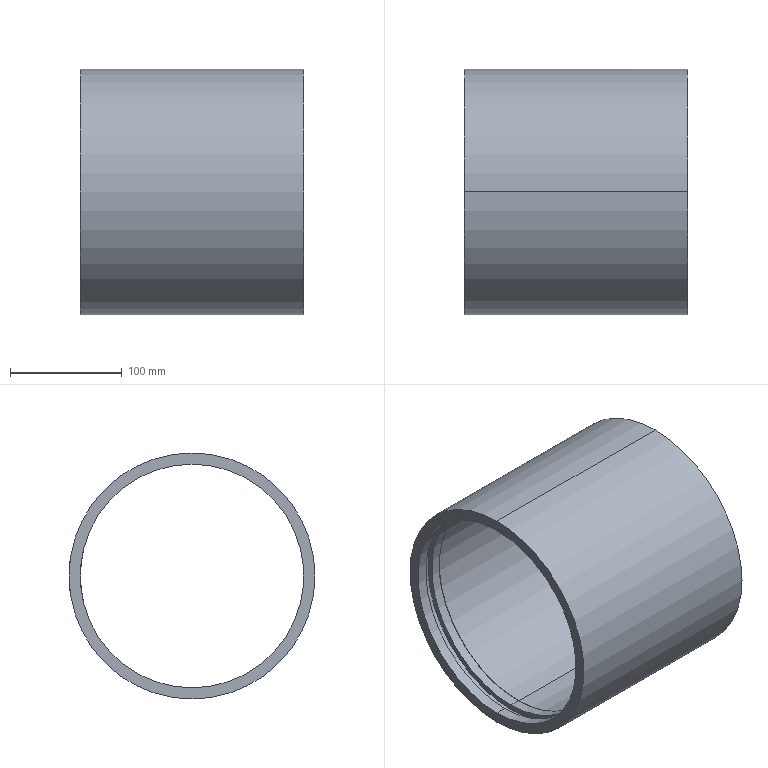Part | SolidWorks | features ICE 2, Revolution 1 | 1 solid | 23 faces | box 200 x 220 x 220 mm | volume 1255193 mm3 | cylinder 16 | plane 7 | commonest cylinder face diameters 200 x6 8.5 x2 14 x2 201 x2 210 x2 220 x2
STEP:
#1=CARTESIAN_POINT('',(106.5,99.91,-4.25));
#2=VERTEX_POINT('',#1);
#3=CARTESIAN_POINT('',(106.5,99.91,4.25));
#4=VERTEX_POINT('',#3);
#5=CARTESIAN_POINT('',(106.5,99.91,-4.25));
#6=CARTESIAN_POINT('',(106.223,99.91,-4.25));
#7=CARTESIAN_POINT('',(105.947,99.911,-4.223));
#8=CARTESIAN_POINT('',(105.399,99.915,-4.114));
#9=CARTESIAN_POINT('',(105.131,99.919,-4.033));
#10=CARTESIAN_POINT('',(104.619,99.927,-3.821));
#11=CARTESIAN_POINT('',(104.373,99.932,-3.69));
#12=CARTESIAN_POINT('',(103.907,99.943,-3.379));
#13=CARTESIAN_POINT('',(103.693,99.949,-3.203));
#14=CARTESIAN_POINT('',(103.301,99.961,-2.812));
#15=CARTESIAN_POINT('',(103.122,99.967,-2.593));
#16=CARTESIAN_POINT('',(102.813,99.978,-2.131));
#17=CARTESIAN_POINT('',(102.682,99.983,-1.887));
#18=CARTESIAN_POINT('',(102.469,99.991,-1.373));
#19=CARTESIAN_POINT('',(102.387,99.994,-1.103));
#20=CARTESIAN_POINT('',(102.278,99.999,-0.5597));
#21=CARTESIAN_POINT('',(102.25,100.,-0.2838));
#22=CARTESIAN_POINT('',(102.25,100.,0.2768));
#23=CARTESIAN_POINT('',(102.277,99.999,0.554));
#24=CARTESIAN_POINT('',(102.385,99.994,1.097));
#25=CARTESIAN_POINT('',(102.466,99.991,1.367));
#26=CARTESIAN_POINT('',(102.679,99.983,1.882));
#27=CARTESIAN_POINT('',(102.81,99.978,2.126));
#28=CARTESIAN_POINT('',(103.118,99.967,2.588));
#29=CARTESIAN_POINT('',(103.297,99.961,2.807));
#30=CARTESIAN_POINT('',(103.689,99.949,3.199));
#31=CARTESIAN_POINT('',(103.903,99.943,3.375));
#32=CARTESIAN_POINT('',(104.366,99.932,3.686));
#33=CARTESIAN_POINT('',(104.614,99.927,3.819));
#34=CARTESIAN_POINT('',(105.125,99.919,4.031));
#35=CARTESIAN_POINT('',(105.392,99.915,4.112));
#36=CARTESIAN_POINT('',(105.942,99.911,4.222));
#37=CARTESIAN_POINT('',(106.219,99.91,4.25));
#38=CARTESIAN_POINT('',(106.5,99.91,4.25));
#39=B_SPLINE_CURVE_WITH_KNOTS('',3,(#5,#6,#7,#8,#9,#10,#11,#12,#13,#14,#15,#16,#17,#18,#19,#20,#21,#22,#23,#24,#25,#26,#27,#28,#29,#30,#31,#32,#33,#34,#35,#36,#37,#38),.UNSPECIFIED.,.F.,.F.,(4,2,2,2,2,2,2,2,2,2,2,2,2,2,2,2,4),(0.01329,0.01412,0.01495,0.01578,0.01661,0.01744,0.01827,0.0191,0.01993,0.02076,0.02159,0.02242,0.02325,0.02408,0.02491,0.02574,0.02657),.UNSPECIFIED.);
#40=EDGE_CURVE('',#2,#4,#39,.T.);
#41=ORIENTED_EDGE('',*,*,#40,.F.);
#42=CARTESIAN_POINT('',(106.5,101.5,-4.25));
#43=VERTEX_POINT('',#42);
#44=CARTESIAN_POINT('',(106.5,93.,-4.25));
#45=DIRECTION('',(0.,1.,0.));
#46=VECTOR('',#45,1000.);
#47=LINE('',#44,#46);
#48=EDGE_CURVE('',#2,#43,#47,.T.);
#49=ORIENTED_EDGE('',*,*,#48,.T.);
#50=CARTESIAN_POINT('',(106.5,101.5,4.25));
#51=VERTEX_POINT('',#50);
#52=CARTESIAN_POINT('',(106.5,101.5,0.));
#53=DIRECTION('',(0.,1.,0.));
#54=DIRECTION('',(0.,0.,1.));
#55=AXIS2_PLACEMENT_3D('',#52,#53,#54);
#56=CIRCLE('',#55,4.25);
#57=EDGE_CURVE('',#43,#51,#56,.T.);
#58=ORIENTED_EDGE('',*,*,#57,.T.);
#59=CARTESIAN_POINT('',(106.5,93.,4.25));
#60=DIRECTION('',(0.,1.,0.));
#61=VECTOR('',#60,1000.);
#62=LINE('',#59,#61);
#63=EDGE_CURVE('',#4,#51,#62,.T.);
#64=ORIENTED_EDGE('',*,*,#63,.F.);
#65=EDGE_LOOP('',(#41,#49,#58,#64));
#66=FACE_OUTER_BOUND('',#65,.T.);
#67=CARTESIAN_POINT('',(106.5,93.,0.));
#68=DIRECTION('',(0.,1.,0.));
#69=DIRECTION('',(0.,0.,1.));
#70=AXIS2_PLACEMENT_3D('',#67,#68,#69);
#71=CYLINDRICAL_SURFACE('',#70,4.25);
#72=ADVANCED_FACE('',(#66),#71,.F.);
#73=CARTESIAN_POINT('',(106.5,101.5,-7.));
#74=VERTEX_POINT('',#73);
#75=CARTESIAN_POINT('',(106.5,101.5,7.));
#76=VERTEX_POINT('',#75);
#77=CARTESIAN_POINT('',(106.5,101.5,0.));
#78=DIRECTION('',(0.,1.,0.));
#79=DIRECTION('',(0.,0.,1.));
#80=AXIS2_PLACEMENT_3D('',#77,#78,#79);
#81=CIRCLE('',#80,7.);
#82=EDGE_CURVE('',#74,#76,#81,.T.);
#83=ORIENTED_EDGE('',*,*,#82,.F.);
#84=CARTESIAN_POINT('',(106.5,109.777,-7.));
#85=VERTEX_POINT('',#84);
#86=CARTESIAN_POINT('',(106.5,101.5,-7.));
#87=DIRECTION('',(0.,1.,0.));
#88=VECTOR('',#87,1000.);
#89=LINE('',#86,#88);
#90=EDGE_CURVE('',#74,#85,#89,.T.);
#91=ORIENTED_EDGE('',*,*,#90,.T.);
#92=CARTESIAN_POINT('',(106.5,109.777,7.));
#93=VERTEX_POINT('',#92);
#94=CARTESIAN_POINT('',(106.5,109.777,7.));
#95=CARTESIAN_POINT('',(106.038,109.777,7.));
#96=CARTESIAN_POINT('',(105.583,109.78,6.955));
#97=CARTESIAN_POINT('',(104.912,109.788,6.821));
#98=CARTESIAN_POINT('',(104.69,109.792,6.766));
#99=CARTESIAN_POINT('',(104.25,109.8,6.632));
#100=CARTESIAN_POINT('',(104.031,109.805,6.554));
#101=CARTESIAN_POINT('',(103.395,109.82,6.291));
#102=CARTESIAN_POINT('',(102.993,109.832,6.075));
#103=CARTESIAN_POINT('',(102.233,109.859,5.567));
#104=CARTESIAN_POINT('',(101.872,109.874,5.272));
#105=CARTESIAN_POINT('',(101.227,109.903,4.626));
#106=CARTESIAN_POINT('',(100.937,109.918,4.274));
#107=CARTESIAN_POINT('',(100.553,109.938,3.7));
#108=CARTESIAN_POINT('',(100.434,109.944,3.501));
#109=CARTESIAN_POINT('',(100.218,109.957,3.097));
#110=CARTESIAN_POINT('',(100.023,109.968,2.684));
#111=CARTESIAN_POINT('',(99.869,109.977,2.254));
#112=CARTESIAN_POINT('',(99.736,109.985,1.816));
#113=CARTESIAN_POINT('',(99.68,109.989,1.591));
#114=CARTESIAN_POINT('',(99.545,109.997,0.9135));
#115=CARTESIAN_POINT('',(99.5,110.,0.4592));
#116=CARTESIAN_POINT('',(99.5,110.,-0.4542));
#117=CARTESIAN_POINT('',(99.546,109.997,-0.9181));
#118=CARTESIAN_POINT('',(99.724,109.986,-1.816));
#119=CARTESIAN_POINT('',(99.857,109.978,-2.252));
#120=CARTESIAN_POINT('',(100.12,109.962,-2.888));
#121=CARTESIAN_POINT('',(100.219,109.957,-3.098));
#122=CARTESIAN_POINT('',(100.436,109.944,-3.503));
#123=CARTESIAN_POINT('',(100.553,109.938,-3.699));
#124=CARTESIAN_POINT('',(100.933,109.918,-4.268));
#125=CARTESIAN_POINT('',(101.223,109.903,-4.622));
#126=CARTESIAN_POINT('',(101.876,109.874,-5.276));
#127=CARTESIAN_POINT('',(102.23,109.859,-5.565));
#128=CARTESIAN_POINT('',(102.799,109.839,-5.946));
#129=CARTESIAN_POINT('',(102.995,109.833,-6.063));
#130=CARTESIAN_POINT('',(103.4,109.821,-6.28));
#131=CARTESIAN_POINT('',(103.609,109.815,-6.379));
#132=CARTESIAN_POINT('',(104.246,109.799,-6.643));
#133=CARTESIAN_POINT('',(104.682,109.791,-6.775));
#134=CARTESIAN_POINT('',(105.579,109.78,-6.954));
#135=CARTESIAN_POINT('',(106.043,109.777,-7.));
#136=CARTESIAN_POINT('',(106.5,109.777,-7.));
#137=B_SPLINE_CURVE_WITH_KNOTS('',3,(#94,#95,#96,#97,#98,#99,#100,#101,#102,#103,#104,#105,#106,#107,#108,#109,#110,#111,#112,#113,#114,#115,#116,#117,#118,#119,#120,#121,#122,#123,#124,#125,#126,#127,#128,#129,#130,#131,#132,#133,#134,#135,#136),.UNSPECIFIED.,.F.,.F.,(4,2,2,2,2,2,2,2,1,2,2,2,2,2,2,2,2,2,2,2,2,4),(0.,0.001368,0.002052,0.002736,0.004105,0.005473,0.006841,0.007525,0.008209,0.008893,0.009577,0.01095,0.01231,0.01368,0.01437,0.01505,0.01642,0.01779,0.01847,0.01915,0.02052,0.02189),.UNSPECIFIED.);
#138=EDGE_CURVE('',#93,#85,#137,.T.);
#139=ORIENTED_EDGE('',*,*,#138,.F.);
#140=CARTESIAN_POINT('',(106.5,101.5,7.));
#141=DIRECTION('',(0.,1.,0.));
#142=VECTOR('',#141,1000.);
#143=LINE('',#140,#142);
#144=EDGE_CURVE('',#76,#93,#143,.T.);
#145=ORIENTED_EDGE('',*,*,#144,.F.);
#146=EDGE_LOOP('',(#83,#91,#139,#145));
#147=FACE_OUTER_BOUND('',#146,.T.);
#148=CARTESIAN_POINT('',(106.5,101.5,0.));
#149=DIRECTION('',(0.,1.,0.));
#150=DIRECTION('',(0.,0.,1.));
#151=AXIS2_PLACEMENT_3D('',#148,#149,#150);
#152=CYLINDRICAL_SURFACE('',#151,7.);
#153=ADVANCED_FACE('',(#147),#152,.F.);
#154=CARTESIAN_POINT('',(-71.,0.,-100.));
#155=VERTEX_POINT('',#154);
#156=CARTESIAN_POINT('',(-71.,0.,100.));
#157=VERTEX_POINT('',#156);
#158=CARTESIAN_POINT('',(-71.,0.,0.));
#159=DIRECTION('',(-1.,0.,0.));
#160=DIRECTION('',(0.,0.,1.));
#161=AXIS2_PLACEMENT_3D('',#158,#159,#160);
#162=CIRCLE('',#161,100.);
#163=EDGE_CURVE('',#155,#157,#162,.T.);
#164=ORIENTED_EDGE('',*,*,#163,.F.);
#165=CARTESIAN_POINT('',(-81.,0.,-100.));
#166=VERTEX_POINT('',#165);
#167=CARTESIAN_POINT('',(-113.63,0.,-100.));
#168=DIRECTION('',(-1.,0.,0.));
#169=VECTOR('',#168,1000.);
#170=LINE('',#167,#169);
#171=EDGE_CURVE('',#155,#166,#170,.T.);
#172=ORIENTED_EDGE('',*,*,#171,.T.);
#173=CARTESIAN_POINT('',(-81.,0.,100.));
#174=VERTEX_POINT('',#173);
#175=CARTESIAN_POINT('',(-81.,0.,0.));
#176=DIRECTION('',(-1.,0.,0.));
#177=DIRECTION('',(0.,0.,1.));
#178=AXIS2_PLACEMENT_3D('',#175,#176,#177);
#179=CIRCLE('',#178,100.);
#180=EDGE_CURVE('',#166,#174,#179,.T.);
#181=ORIENTED_EDGE('',*,*,#180,.T.);
#182=CARTESIAN_POINT('',(-113.63,0.,100.));
#183=DIRECTION('',(-1.,0.,0.));
#184=VECTOR('',#183,1000.);
#185=LINE('',#182,#184);
#186=EDGE_CURVE('',#157,#174,#185,.T.);
#187=ORIENTED_EDGE('',*,*,#186,.F.);
#188=EDGE_LOOP('',(#164,#172,#181,#187));
#189=FACE_OUTER_BOUND('',#188,.T.);
#190=CARTESIAN_POINT('',(-113.63,0.,0.));
#191=DIRECTION('',(-1.,0.,0.));
#192=DIRECTION('',(0.,0.,1.));
#193=AXIS2_PLACEMENT_3D('',#190,#191,#192);
#194=CYLINDRICAL_SURFACE('',#193,100.);
#195=ADVANCED_FACE('',(#189),#194,.F.);
#196=CARTESIAN_POINT('',(-63.5,0.,-105.));
#197=VERTEX_POINT('',#196);
#198=CARTESIAN_POINT('',(-63.5,0.,105.));
#199=VERTEX_POINT('',#198);
#200=CARTESIAN_POINT('',(-63.5,0.,0.));
#201=DIRECTION('',(-1.,0.,0.));
#202=DIRECTION('',(0.,0.,1.));
#203=AXIS2_PLACEMENT_3D('',#200,#201,#202);
#204=CIRCLE('',#203,105.);
#205=EDGE_CURVE('',#197,#199,#204,.T.);
#206=ORIENTED_EDGE('',*,*,#205,.F.);
#207=CARTESIAN_POINT('',(-71.,0.,-105.));
#208=VERTEX_POINT('',#207);
#209=CARTESIAN_POINT('',(-113.63,0.,-105.));
#210=DIRECTION('',(-1.,0.,0.));
#211=VECTOR('',#210,1000.);
#212=LINE('',#209,#211);
#213=EDGE_CURVE('',#197,#208,#212,.T.);
#214=ORIENTED_EDGE('',*,*,#213,.T.);
#215=CARTESIAN_POINT('',(-71.,0.,105.));
#216=VERTEX_POINT('',#215);
#217=CARTESIAN_POINT('',(-71.,0.,0.));
#218=DIRECTION('',(-1.,0.,0.));
#219=DIRECTION('',(0.,0.,1.));
#220=AXIS2_PLACEMENT_3D('',#217,#218,#219);
#221=CIRCLE('',#220,105.);
#222=EDGE_CURVE('',#208,#216,#221,.T.);
#223=ORIENTED_EDGE('',*,*,#222,.T.);
#224=CARTESIAN_POINT('',(-113.63,0.,105.));
#225=DIRECTION('',(-1.,0.,0.));
#226=VECTOR('',#225,1000.);
#227=LINE('',#224,#226);
#228=EDGE_CURVE('',#199,#216,#227,.T.);
#229=ORIENTED_EDGE('',*,*,#228,.F.);
#230=EDGE_LOOP('',(#206,#214,#223,#229));
#231=FACE_OUTER_BOUND('',#230,.T.);
#232=CARTESIAN_POINT('',(-113.63,0.,0.));
#233=DIRECTION('',(-1.,0.,0.));
#234=DIRECTION('',(0.,0.,1.));
#235=AXIS2_PLACEMENT_3D('',#232,#233,#234);
#236=CYLINDRICAL_SURFACE('',#235,105.);
#237=ADVANCED_FACE('',(#231),#236,.F.);
#238=CARTESIAN_POINT('',(-54.,0.,-100.));
#239=VERTEX_POINT('',#238);
#240=CARTESIAN_POINT('',(-54.,0.,100.));
#241=VERTEX_POINT('',#240);
#242=CARTESIAN_POINT('',(-54.,0.,0.));
#243=DIRECTION('',(-1.,0.,0.));
#244=DIRECTION('',(0.,0.,1.));
#245=AXIS2_PLACEMENT_3D('',#242,#243,#244);
#246=CIRCLE('',#245,100.);
#247=EDGE_CURVE('',#239,#241,#246,.T.);
#248=ORIENTED_EDGE('',*,*,#247,.F.);
#249=CARTESIAN_POINT('',(-63.5,0.,-100.));
#250=VERTEX_POINT('',#249);
#251=CARTESIAN_POINT('',(-113.63,0.,-100.));
#252=DIRECTION('',(-1.,0.,0.));
#253=VECTOR('',#252,1000.);
#254=LINE('',#251,#253);
#255=EDGE_CURVE('',#239,#250,#254,.T.);
#256=ORIENTED_EDGE('',*,*,#255,.T.);
#257=CARTESIAN_POINT('',(-63.5,0.,100.));
#258=VERTEX_POINT('',#257);
#259=CARTESIAN_POINT('',(-63.5,0.,0.));
#260=DIRECTION('',(-1.,0.,0.));
#261=DIRECTION('',(0.,0.,1.));
#262=AXIS2_PLACEMENT_3D('',#259,#260,#261);
#263=CIRCLE('',#262,100.);
#264=EDGE_CURVE('',#250,#258,#263,.T.);
#265=ORIENTED_EDGE('',*,*,#264,.T.);
#266=CARTESIAN_POINT('',(-113.63,0.,100.));
#267=DIRECTION('',(-1.,0.,0.));
#268=VECTOR('',#267,1000.);
#269=LINE('',#266,#268);
#270=EDGE_CURVE('',#241,#258,#269,.T.);
#271=ORIENTED_EDGE('',*,*,#270,.F.);
#272=EDGE_LOOP('',(#248,#256,#265,#271));
#273=FACE_OUTER_BOUND('',#272,.T.);
#274=CARTESIAN_POINT('',(-113.63,0.,0.));
#275=DIRECTION('',(-1.,0.,0.));
#276=DIRECTION('',(0.,0.,1.));
#277=AXIS2_PLACEMENT_3D('',#274,#275,#276);
#278=CYLINDRICAL_SURFACE('',#277,100.);
#279=ADVANCED_FACE('',(#273),#278,.F.);
#280=CARTESIAN_POINT('',(69.,0.,-100.5));
#281=VERTEX_POINT('',#280);
#282=CARTESIAN_POINT('',(69.,0.,100.5));
#283=VERTEX_POINT('',#282);
#284=CARTESIAN_POINT('',(69.,0.,0.));
#285=DIRECTION('',(-1.,0.,0.));
#286=DIRECTION('',(0.,0.,1.));
#287=AXIS2_PLACEMENT_3D('',#284,#285,#286);
#288=CIRCLE('',#287,100.5);
#289=EDGE_CURVE('',#281,#283,#288,.T.);
#290=ORIENTED_EDGE('',*,*,#289,.F.);
#291=CARTESIAN_POINT('',(-54.,0.,-100.5));
#292=VERTEX_POINT('',#291);
#293=CARTESIAN_POINT('',(-113.63,0.,-100.5));
#294=DIRECTION('',(-1.,0.,0.));
#295=VECTOR('',#294,1000.);
#296=LINE('',#293,#295);
#297=EDGE_CURVE('',#281,#292,#296,.T.);
#298=ORIENTED_EDGE('',*,*,#297,.T.);
#299=CARTESIAN_POINT('',(-54.,0.,100.5));
#300=VERTEX_POINT('',#299);
#301=CARTESIAN_POINT('',(-54.,0.,0.));
#302=DIRECTION('',(-1.,0.,0.));
#303=DIRECTION('',(0.,0.,1.));
#304=AXIS2_PLACEMENT_3D('',#301,#302,#303);
#305=CIRCLE('',#304,100.5);
#306=EDGE_CURVE('',#292,#300,#305,.T.);
#307=ORIENTED_EDGE('',*,*,#306,.T.);
#308=CARTESIAN_POINT('',(-113.63,0.,100.5));
#309=DIRECTION('',(-1.,0.,0.));
#310=VECTOR('',#309,1000.);
#311=LINE('',#308,#310);
#312=EDGE_CURVE('',#283,#300,#311,.T.);
#313=ORIENTED_EDGE('',*,*,#312,.F.);
#314=EDGE_LOOP('',(#290,#298,#307,#313));
#315=FACE_OUTER_BOUND('',#314,.T.);
#316=CARTESIAN_POINT('',(-113.63,0.,0.));
#317=DIRECTION('',(-1.,0.,0.));
#318=DIRECTION('',(0.,0.,1.));
#319=AXIS2_PLACEMENT_3D('',#316,#317,#318);
#320=CYLINDRICAL_SURFACE('',#319,100.5);
#321=ADVANCED_FACE('',(#315),#320,.F.);
#322=CARTESIAN_POINT('',(119.,0.,-100.));
#323=VERTEX_POINT('',#322);
#324=CARTESIAN_POINT('',(119.,0.,100.));
#325=VERTEX_POINT('',#324);
#326=CARTESIAN_POINT('',(119.,0.,0.));
#327=DIRECTION('',(-1.,0.,0.));
#328=DIRECTION('',(0.,0.,1.));
#329=AXIS2_PLACEMENT_3D('',#326,#327,#328);
#330=CIRCLE('',#329,100.);
#331=EDGE_CURVE('',#323,#325,#330,.T.);
#332=ORIENTED_EDGE('',*,*,#331,.F.);
#333=CARTESIAN_POINT('',(69.,0.,-100.));
#334=VERTEX_POINT('',#333);
#335=CARTESIAN_POINT('',(-113.63,0.,-100.));
#336=DIRECTION('',(-1.,0.,0.));
#337=VECTOR('',#336,1000.);
#338=LINE('',#335,#337);
#339=EDGE_CURVE('',#323,#334,#338,.T.);
#340=ORIENTED_EDGE('',*,*,#339,.T.);
#341=CARTESIAN_POINT('',(69.,0.,100.));
#342=VERTEX_POINT('',#341);
#343=CARTESIAN_POINT('',(69.,0.,0.));
#344=DIRECTION('',(-1.,0.,0.));
#345=DIRECTION('',(0.,0.,1.));
#346=AXIS2_PLACEMENT_3D('',#343,#344,#345);
#347=CIRCLE('',#346,100.);
#348=EDGE_CURVE('',#334,#342,#347,.T.);
#349=ORIENTED_EDGE('',*,*,#348,.T.);
#350=CARTESIAN_POINT('',(-113.63,0.,100.));
#351=DIRECTION('',(-1.,0.,0.));
#352=VECTOR('',#351,1000.);
#353=LINE('',#350,#352);
#354=EDGE_CURVE('',#325,#342,#353,.T.);
#355=ORIENTED_EDGE('',*,*,#354,.F.);
#356=EDGE_LOOP('',(#332,#340,#349,#355));
#357=FACE_OUTER_BOUND('',#356,.T.);
#358=CARTESIAN_POINT('',(-113.63,0.,0.));
#359=DIRECTION('',(-1.,0.,0.));
#360=DIRECTION('',(0.,0.,1.));
#361=AXIS2_PLACEMENT_3D('',#358,#359,#360);
#362=CYLINDRICAL_SURFACE('',#361,100.);
#363=ADVANCED_FACE('',(#357),#362,.F.);
#364=ORIENTED_EDGE('',*,*,#138,.T.);
#365=CARTESIAN_POINT('',(106.5,109.777,-7.));
#366=CARTESIAN_POINT('',(106.957,109.777,-7.));
#367=CARTESIAN_POINT('',(107.411,109.78,-6.956));
#368=CARTESIAN_POINT('',(108.088,109.788,-6.821));
#369=CARTESIAN_POINT('',(108.313,109.792,-6.765));
#370=CARTESIAN_POINT('',(108.752,109.8,-6.632));
#371=CARTESIAN_POINT('',(109.182,109.809,-6.478));
#372=CARTESIAN_POINT('',(109.594,109.82,-6.283));
#373=CARTESIAN_POINT('',(109.998,109.833,-6.068));
#374=CARTESIAN_POINT('',(110.196,109.839,-5.949));
#375=CARTESIAN_POINT('',(110.771,109.859,-5.565));
#376=CARTESIAN_POINT('',(111.124,109.874,-5.276));
#377=CARTESIAN_POINT('',(111.769,109.903,-4.631));
#378=CARTESIAN_POINT('',(112.065,109.918,-4.271));
#379=CARTESIAN_POINT('',(112.574,109.945,-3.51));
#380=CARTESIAN_POINT('',(112.789,109.957,-3.108));
#381=CARTESIAN_POINT('',(113.053,109.972,-2.473));
#382=CARTESIAN_POINT('',(113.131,109.977,-2.255));
#383=CARTESIAN_POINT('',(113.265,109.985,-1.815));
#384=CARTESIAN_POINT('',(113.32,109.989,-1.593));
#385=CARTESIAN_POINT('',(113.454,109.997,-0.9221));
#386=CARTESIAN_POINT('',(113.5,110.,-0.4676));
#387=CARTESIAN_POINT('',(113.501,110.,0.4562));
#388=CARTESIAN_POINT('',(113.455,109.997,0.9125));
#389=CARTESIAN_POINT('',(113.323,109.989,1.583));
#390=CARTESIAN_POINT('',(113.267,109.985,1.805));
#391=CARTESIAN_POINT('',(113.135,109.977,2.245));
#392=CARTESIAN_POINT('',(113.057,109.973,2.463));
#393=CARTESIAN_POINT('',(112.793,109.957,3.1));
#394=CARTESIAN_POINT('',(112.578,109.945,3.502));
#395=CARTESIAN_POINT('',(112.072,109.918,4.263));
#396=CARTESIAN_POINT('',(111.776,109.903,4.623));
#397=CARTESIAN_POINT('',(111.131,109.874,5.269));
#398=CARTESIAN_POINT('',(110.779,109.86,5.559));
#399=CARTESIAN_POINT('',(110.206,109.839,5.943));
#400=CARTESIAN_POINT('',(110.007,109.833,6.063));
#401=CARTESIAN_POINT('',(109.603,109.821,6.279));
#402=CARTESIAN_POINT('',(109.397,109.815,6.377));
#403=CARTESIAN_POINT('',(108.765,109.8,6.639));
#404=CARTESIAN_POINT('',(108.326,109.791,6.774));
#405=CARTESIAN_POINT('',(107.42,109.78,6.955));
#406=CARTESIAN_POINT('',(106.963,109.777,7.));
#407=CARTESIAN_POINT('',(106.5,109.777,7.));
#408=B_SPLINE_CURVE_WITH_KNOTS('',3,(#365,#366,#367,#368,#369,#370,#371,#372,#373,#374,#375,#376,#377,#378,#379,#380,#381,#382,#383,#384,#385,#386,#387,#388,#389,#390,#391,#392,#393,#394,#395,#396,#397,#398,#399,#400,#401,#402,#403,#404,#405,#406,#407),.UNSPECIFIED.,.F.,.F.,(4,2,2,1,2,2,2,2,2,2,2,2,2,2,2,2,2,2,2,2,2,4),(0.02189,0.02326,0.02394,0.02463,0.02531,0.02599,0.02736,0.02873,0.0301,0.03078,0.03147,0.03283,0.0342,0.03489,0.03557,0.03694,0.0383,0.03967,0.04036,0.04104,0.04241,0.04378),.UNSPECIFIED.);
#409=EDGE_CURVE('',#85,#93,#408,.T.);
#410=ORIENTED_EDGE('',*,*,#409,.T.);
#411=EDGE_LOOP('',(#364,#410));
#412=FACE_BOUND('',#411,.T.);
#413=CARTESIAN_POINT('',(119.,0.,110.));
#414=VERTEX_POINT('',#413);
#415=CARTESIAN_POINT('',(119.,0.,-110.));
#416=VERTEX_POINT('',#415);
#417=CARTESIAN_POINT('',(119.,0.,0.));
#418=DIRECTION('',(-1.,0.,0.));
#419=DIRECTION('',(0.,0.,1.));
#420=AXIS2_PLACEMENT_3D('',#417,#418,#419);
#421=CIRCLE('',#420,110.);
#422=EDGE_CURVE('',#414,#416,#421,.T.);
#423=ORIENTED_EDGE('',*,*,#422,.T.);
#424=CARTESIAN_POINT('',(-81.,0.,-110.));
#425=VERTEX_POINT('',#424);
#426=CARTESIAN_POINT('',(-113.63,0.,-110.));
#427=DIRECTION('',(-1.,0.,0.));
#428=VECTOR('',#427,1000.);
#429=LINE('',#426,#428);
#430=EDGE_CURVE('',#416,#425,#429,.T.);
#431=ORIENTED_EDGE('',*,*,#430,.T.);
#432=CARTESIAN_POINT('',(-81.,0.,110.));
#433=VERTEX_POINT('',#432);
#434=CARTESIAN_POINT('',(-81.,0.,0.));
#435=DIRECTION('',(-1.,0.,0.));
#436=DIRECTION('',(0.,0.,1.));
#437=AXIS2_PLACEMENT_3D('',#434,#435,#436);
#438=CIRCLE('',#437,110.);
#439=EDGE_CURVE('',#433,#425,#438,.T.);
#440=ORIENTED_EDGE('',*,*,#439,.F.);
#441=CARTESIAN_POINT('',(-113.63,0.,110.));
#442=DIRECTION('',(-1.,0.,0.));
#443=VECTOR('',#442,1000.);
#444=LINE('',#441,#443);
#445=EDGE_CURVE('',#414,#433,#444,.T.);
#446=ORIENTED_EDGE('',*,*,#445,.F.);
#447=EDGE_LOOP('',(#423,#431,#440,#446));
#448=FACE_OUTER_BOUND('',#447,.T.);
#449=CARTESIAN_POINT('',(-113.63,0.,0.));
#450=DIRECTION('',(-1.,0.,0.));
#451=DIRECTION('',(0.,0.,1.));
#452=AXIS2_PLACEMENT_3D('',#449,#450,#451);
#453=CYLINDRICAL_SURFACE('',#452,110.);
#454=ADVANCED_FACE('',(#412,#448),#453,.T.);
#455=ORIENTED_EDGE('',*,*,#430,.F.);
#456=CARTESIAN_POINT('',(119.,0.,0.));
#457=DIRECTION('',(-1.,0.,0.));
#458=DIRECTION('',(0.,0.,1.));
#459=AXIS2_PLACEMENT_3D('',#456,#457,#458);
#460=CIRCLE('',#459,110.);
#461=EDGE_CURVE('',#416,#414,#460,.T.);
#462=ORIENTED_EDGE('',*,*,#461,.T.);
#463=ORIENTED_EDGE('',*,*,#445,.T.);
#464=CARTESIAN_POINT('',(-81.,0.,0.));
#465=DIRECTION('',(-1.,0.,0.));
#466=DIRECTION('',(0.,0.,1.));
#467=AXIS2_PLACEMENT_3D('',#464,#465,#466);
#468=CIRCLE('',#467,110.);
#469=EDGE_CURVE('',#425,#433,#468,.T.);
#470=ORIENTED_EDGE('',*,*,#469,.F.);
#471=EDGE_LOOP('',(#455,#462,#463,#470));
#472=FACE_OUTER_BOUND('',#471,.T.);
#473=CARTESIAN_POINT('',(-113.63,0.,0.));
#474=DIRECTION('',(-1.,0.,0.));
#475=DIRECTION('',(0.,0.,1.));
#476=AXIS2_PLACEMENT_3D('',#473,#474,#475);
#477=CYLINDRICAL_SURFACE('',#476,110.);
#478=ADVANCED_FACE('',(#472),#477,.T.);
#479=ORIENTED_EDGE('',*,*,#422,.F.);
#480=ORIENTED_EDGE('',*,*,#461,.F.);
#481=EDGE_LOOP('',(#479,#480));
#482=FACE_OUTER_BOUND('',#481,.T.);
#483=CARTESIAN_POINT('',(119.,0.,0.));
#484=DIRECTION('',(-1.,0.,0.));
#485=DIRECTION('',(0.,0.,1.));
#486=AXIS2_PLACEMENT_3D('',#483,#484,#485);
#487=CIRCLE('',#486,100.);
#488=EDGE_CURVE('',#325,#323,#487,.T.);
#489=ORIENTED_EDGE('',*,*,#488,.T.);
#490=ORIENTED_EDGE('',*,*,#331,.T.);
#491=EDGE_LOOP('',(#489,#490));
#492=FACE_BOUND('',#491,.T.);
#493=CARTESIAN_POINT('',(119.,110.,0.));
#494=DIRECTION('',(-1.,0.,0.));
#495=DIRECTION('',(0.,0.,1.));
#496=AXIS2_PLACEMENT_3D('',#493,#494,#495);
#497=PLANE('',#496);
#498=ADVANCED_FACE('',(#482,#492),#497,.F.);
#499=ORIENTED_EDGE('',*,*,#339,.F.);
#500=ORIENTED_EDGE('',*,*,#488,.F.);
#501=ORIENTED_EDGE('',*,*,#354,.T.);
#502=CARTESIAN_POINT('',(69.,0.,0.));
#503=DIRECTION('',(-1.,0.,0.));
#504=DIRECTION('',(0.,0.,1.));
#505=AXIS2_PLACEMENT_3D('',#502,#503,#504);
#506=CIRCLE('',#505,100.);
#507=EDGE_CURVE('',#342,#334,#506,.T.);
#508=ORIENTED_EDGE('',*,*,#507,.T.);
#509=EDGE_LOOP('',(#499,#500,#501,#508));
#510=FACE_OUTER_BOUND('',#509,.T.);
#511=CARTESIAN_POINT('',(106.5,99.91,4.25));
#512=CARTESIAN_POINT('',(106.781,99.91,4.25));
#513=CARTESIAN_POINT('',(107.057,99.911,4.222));
#514=CARTESIAN_POINT('',(107.6,99.915,4.114));
#515=CARTESIAN_POINT('',(107.87,99.919,4.033));
#516=CARTESIAN_POINT('',(108.385,99.927,3.819));
#517=CARTESIAN_POINT('',(108.629,99.932,3.689));
#518=CARTESIAN_POINT('',(109.091,99.943,3.38));
#519=CARTESIAN_POINT('',(109.31,99.949,3.201));
#520=CARTESIAN_POINT('',(109.702,99.961,2.809));
#521=CARTESIAN_POINT('',(109.878,99.967,2.595));
#522=CARTESIAN_POINT('',(110.189,99.978,2.13));
#523=CARTESIAN_POINT('',(110.321,99.983,1.883));
#524=CARTESIAN_POINT('',(110.533,99.991,1.371));
#525=CARTESIAN_POINT('',(110.614,99.994,1.103));
#526=CARTESIAN_POINT('',(110.723,99.999,0.5546));
#527=CARTESIAN_POINT('',(110.75,100.,0.2787));
#528=CARTESIAN_POINT('',(110.75,100.,-0.2757));
#529=CARTESIAN_POINT('',(110.723,99.999,-0.5573));
#530=CARTESIAN_POINT('',(110.614,99.994,-1.102));
#531=CARTESIAN_POINT('',(110.534,99.991,-1.367));
#532=CARTESIAN_POINT('',(110.321,99.983,-1.882));
#533=CARTESIAN_POINT('',(110.188,99.978,-2.131));
#534=CARTESIAN_POINT('',(109.88,99.967,-2.591));
#535=CARTESIAN_POINT('',(109.704,99.961,-2.806));
#536=CARTESIAN_POINT('',(109.308,99.949,-3.203));
#537=CARTESIAN_POINT('',(109.093,99.943,-3.379));
#538=CARTESIAN_POINT('',(108.632,99.932,-3.687));
#539=CARTESIAN_POINT('',(108.384,99.927,-3.82));
#540=CARTESIAN_POINT('',(107.869,99.919,-4.033));
#541=CARTESIAN_POINT('',(107.604,99.915,-4.114));
#542=CARTESIAN_POINT('',(107.059,99.911,-4.222));
#543=CARTESIAN_POINT('',(106.778,99.91,-4.25));
#544=CARTESIAN_POINT('',(106.5,99.91,-4.25));
#545=B_SPLINE_CURVE_WITH_KNOTS('',3,(#511,#512,#513,#514,#515,#516,#517,#518,#519,#520,#521,#522,#523,#524,#525,#526,#527,#528,#529,#530,#531,#532,#533,#534,#535,#536,#537,#538,#539,#540,#541,#542,#543,#544),.UNSPECIFIED.,.F.,.F.,(4,2,2,2,2,2,2,2,2,2,2,2,2,2,2,2,4),(0.,0.0008306,0.001661,0.002492,0.003322,0.004153,0.004983,0.005814,0.006644,0.007475,0.008306,0.009136,0.009967,0.0108,0.01163,0.01246,0.01329),.UNSPECIFIED.);
#546=EDGE_CURVE('',#4,#2,#545,.T.);
#547=ORIENTED_EDGE('',*,*,#546,.T.);
#548=ORIENTED_EDGE('',*,*,#40,.T.);
#549=EDGE_LOOP('',(#547,#548));
#550=FACE_BOUND('',#549,.T.);
#551=CARTESIAN_POINT('',(-113.63,0.,0.));
#552=DIRECTION('',(-1.,0.,0.));
#553=DIRECTION('',(0.,0.,1.));
#554=AXIS2_PLACEMENT_3D('',#551,#552,#553);
#555=CYLINDRICAL_SURFACE('',#554,100.);
#556=ADVANCED_FACE('',(#510,#550),#555,.F.);
#557=ORIENTED_EDGE('',*,*,#507,.F.);
#558=ORIENTED_EDGE('',*,*,#348,.F.);
#559=EDGE_LOOP('',(#557,#558));
#560=FACE_BOUND('',#559,.T.);
#561=CARTESIAN_POINT('',(69.,0.,0.));
#562=DIRECTION('',(-1.,0.,0.));
#563=DIRECTION('',(0.,0.,1.));
#564=AXIS2_PLACEMENT_3D('',#561,#562,#563);
#565=CIRCLE('',#564,100.5);
#566=EDGE_CURVE('',#283,#281,#565,.T.);
#567=ORIENTED_EDGE('',*,*,#566,.T.);
#568=ORIENTED_EDGE('',*,*,#289,.T.);
#569=EDGE_LOOP('',(#567,#568));
#570=FACE_OUTER_BOUND('',#569,.T.);
#571=CARTESIAN_POINT('',(69.,100.,0.));
#572=DIRECTION('',(1.,0.,0.));
#573=DIRECTION('',(0.,0.,-1.));
#574=AXIS2_PLACEMENT_3D('',#571,#572,#573);
#575=PLANE('',#574);
#576=ADVANCED_FACE('',(#560,#570),#575,.F.);
#577=ORIENTED_EDGE('',*,*,#297,.F.);
#578=ORIENTED_EDGE('',*,*,#566,.F.);
#579=ORIENTED_EDGE('',*,*,#312,.T.);
#580=CARTESIAN_POINT('',(-54.,0.,0.));
#581=DIRECTION('',(-1.,0.,0.));
#582=DIRECTION('',(0.,0.,1.));
#583=AXIS2_PLACEMENT_3D('',#580,#581,#582);
#584=CIRCLE('',#583,100.5);
#585=EDGE_CURVE('',#300,#292,#584,.T.);
#586=ORIENTED_EDGE('',*,*,#585,.T.);
#587=EDGE_LOOP('',(#577,#578,#579,#586));
#588=FACE_OUTER_BOUND('',#587,.T.);
#589=CARTESIAN_POINT('',(-113.63,0.,0.));
#590=DIRECTION('',(-1.,0.,0.));
#591=DIRECTION('',(0.,0.,1.));
#592=AXIS2_PLACEMENT_3D('',#589,#590,#591);
#593=CYLINDRICAL_SURFACE('',#592,100.5);
#594=ADVANCED_FACE('',(#588),#593,.F.);
#595=ORIENTED_EDGE('',*,*,#585,.F.);
#596=ORIENTED_EDGE('',*,*,#306,.F.);
#597=EDGE_LOOP('',(#595,#596));
#598=FACE_OUTER_BOUND('',#597,.T.);
#599=CARTESIAN_POINT('',(-54.,0.,0.));
#600=DIRECTION('',(-1.,0.,0.));
#601=DIRECTION('',(0.,0.,1.));
#602=AXIS2_PLACEMENT_3D('',#599,#600,#601);
#603=CIRCLE('',#602,100.);
#604=EDGE_CURVE('',#241,#239,#603,.T.);
#605=ORIENTED_EDGE('',*,*,#604,.T.);
#606=ORIENTED_EDGE('',*,*,#247,.T.);
#607=EDGE_LOOP('',(#605,#606));
#608=FACE_BOUND('',#607,.T.);
#609=CARTESIAN_POINT('',(-54.,100.5,0.));
#610=DIRECTION('',(-1.,0.,0.));
#611=DIRECTION('',(0.,0.,1.));
#612=AXIS2_PLACEMENT_3D('',#609,#610,#611);
#613=PLANE('',#612);
#614=ADVANCED_FACE('',(#598,#608),#613,.F.);
#615=ORIENTED_EDGE('',*,*,#255,.F.);
#616=ORIENTED_EDGE('',*,*,#604,.F.);
#617=ORIENTED_EDGE('',*,*,#270,.T.);
#618=CARTESIAN_POINT('',(-63.5,0.,0.));
#619=DIRECTION('',(-1.,0.,0.));
#620=DIRECTION('',(0.,0.,1.));
#621=AXIS2_PLACEMENT_3D('',#618,#619,#620);
#622=CIRCLE('',#621,100.);
#623=EDGE_CURVE('',#258,#250,#622,.T.);
#624=ORIENTED_EDGE('',*,*,#623,.T.);
#625=EDGE_LOOP('',(#615,#616,#617,#624));
#626=FACE_OUTER_BOUND('',#625,.T.);
#627=CARTESIAN_POINT('',(-113.63,0.,0.));
#628=DIRECTION('',(-1.,0.,0.));
#629=DIRECTION('',(0.,0.,1.));
#630=AXIS2_PLACEMENT_3D('',#627,#628,#629);
#631=CYLINDRICAL_SURFACE('',#630,100.);
#632=ADVANCED_FACE('',(#626),#631,.F.);
#633=ORIENTED_EDGE('',*,*,#623,.F.);
#634=ORIENTED_EDGE('',*,*,#264,.F.);
#635=EDGE_LOOP('',(#633,#634));
#636=FACE_BOUND('',#635,.T.);
#637=CARTESIAN_POINT('',(-63.5,0.,0.));
#638=DIRECTION('',(-1.,0.,0.));
#639=DIRECTION('',(0.,0.,1.));
#640=AXIS2_PLACEMENT_3D('',#637,#638,#639);
#641=CIRCLE('',#640,105.);
#642=EDGE_CURVE('',#199,#197,#641,.T.);
#643=ORIENTED_EDGE('',*,*,#642,.T.);
#644=ORIENTED_EDGE('',*,*,#205,.T.);
#645=EDGE_LOOP('',(#643,#644));
#646=FACE_OUTER_BOUND('',#645,.T.);
#647=CARTESIAN_POINT('',(-63.5,100.,0.));
#648=DIRECTION('',(1.,0.,0.));
#649=DIRECTION('',(0.,0.,-1.));
#650=AXIS2_PLACEMENT_3D('',#647,#648,#649);
#651=PLANE('',#650);
#652=ADVANCED_FACE('',(#636,#646),#651,.F.);
#653=ORIENTED_EDGE('',*,*,#213,.F.);
#654=ORIENTED_EDGE('',*,*,#642,.F.);
#655=ORIENTED_EDGE('',*,*,#228,.T.);
#656=CARTESIAN_POINT('',(-71.,0.,0.));
#657=DIRECTION('',(-1.,0.,0.));
#658=DIRECTION('',(0.,0.,1.));
#659=AXIS2_PLACEMENT_3D('',#656,#657,#658);
#660=CIRCLE('',#659,105.);
#661=EDGE_CURVE('',#216,#208,#660,.T.);
#662=ORIENTED_EDGE('',*,*,#661,.T.);
#663=EDGE_LOOP('',(#653,#654,#655,#662));
#664=FACE_OUTER_BOUND('',#663,.T.);
#665=CARTESIAN_POINT('',(-113.63,0.,0.));
#666=DIRECTION('',(-1.,0.,0.));
#667=DIRECTION('',(0.,0.,1.));
#668=AXIS2_PLACEMENT_3D('',#665,#666,#667);
#669=CYLINDRICAL_SURFACE('',#668,105.);
#670=ADVANCED_FACE('',(#664),#669,.F.);
#671=ORIENTED_EDGE('',*,*,#661,.F.);
#672=ORIENTED_EDGE('',*,*,#222,.F.);
#673=EDGE_LOOP('',(#671,#672));
#674=FACE_OUTER_BOUND('',#673,.T.);
#675=CARTESIAN_POINT('',(-71.,0.,0.));
#676=DIRECTION('',(-1.,0.,0.));
#677=DIRECTION('',(0.,0.,1.));
#678=AXIS2_PLACEMENT_3D('',#675,#676,#677);
#679=CIRCLE('',#678,100.);
#680=EDGE_CURVE('',#157,#155,#679,.T.);
#681=ORIENTED_EDGE('',*,*,#680,.T.);
#682=ORIENTED_EDGE('',*,*,#163,.T.);
#683=EDGE_LOOP('',(#681,#682));
#684=FACE_BOUND('',#683,.T.);
#685=CARTESIAN_POINT('',(-71.,105.,0.));
#686=DIRECTION('',(-1.,0.,0.));
#687=DIRECTION('',(0.,0.,1.));
#688=AXIS2_PLACEMENT_3D('',#685,#686,#687);
#689=PLANE('',#688);
#690=ADVANCED_FACE('',(#674,#684),#689,.F.);
#691=ORIENTED_EDGE('',*,*,#171,.F.);
#692=ORIENTED_EDGE('',*,*,#680,.F.);
#693=ORIENTED_EDGE('',*,*,#186,.T.);
#694=CARTESIAN_POINT('',(-81.,0.,0.));
#695=DIRECTION('',(-1.,0.,0.));
#696=DIRECTION('',(0.,0.,1.));
#697=AXIS2_PLACEMENT_3D('',#694,#695,#696);
#698=CIRCLE('',#697,100.);
#699=EDGE_CURVE('',#174,#166,#698,.T.);
#700=ORIENTED_EDGE('',*,*,#699,.T.);
#701=EDGE_LOOP('',(#691,#692,#693,#700));
#702=FACE_OUTER_BOUND('',#701,.T.);
#703=CARTESIAN_POINT('',(-113.63,0.,0.));
#704=DIRECTION('',(-1.,0.,0.));
#705=DIRECTION('',(0.,0.,1.));
#706=AXIS2_PLACEMENT_3D('',#703,#704,#705);
#707=CYLINDRICAL_SURFACE('',#706,100.);
#708=ADVANCED_FACE('',(#702),#707,.F.);
#709=ORIENTED_EDGE('',*,*,#699,.F.);
#710=ORIENTED_EDGE('',*,*,#180,.F.);
#711=EDGE_LOOP('',(#709,#710));
#712=FACE_BOUND('',#711,.T.);
#713=ORIENTED_EDGE('',*,*,#439,.T.);
#714=ORIENTED_EDGE('',*,*,#469,.T.);
#715=EDGE_LOOP('',(#713,#714));
#716=FACE_OUTER_BOUND('',#715,.T.);
#717=CARTESIAN_POINT('',(-81.,110.,0.));
#718=DIRECTION('',(1.,0.,0.));
#719=DIRECTION('',(0.,0.,-1.));
#720=AXIS2_PLACEMENT_3D('',#717,#718,#719);
#721=PLANE('',#720);
#722=ADVANCED_FACE('',(#712,#716),#721,.F.);
#723=ORIENTED_EDGE('',*,*,#90,.F.);
#724=CARTESIAN_POINT('',(106.5,101.5,0.));
#725=DIRECTION('',(0.,1.,0.));
#726=DIRECTION('',(0.,0.,1.));
#727=AXIS2_PLACEMENT_3D('',#724,#725,#726);
#728=CIRCLE('',#727,7.);
#729=EDGE_CURVE('',#76,#74,#728,.T.);
#730=ORIENTED_EDGE('',*,*,#729,.F.);
#731=ORIENTED_EDGE('',*,*,#144,.T.);
#732=ORIENTED_EDGE('',*,*,#409,.F.);
#733=EDGE_LOOP('',(#723,#730,#731,#732));
#734=FACE_OUTER_BOUND('',#733,.T.);
#735=CARTESIAN_POINT('',(106.5,101.5,0.));
#736=DIRECTION('',(0.,1.,0.));
#737=DIRECTION('',(0.,0.,1.));
#738=AXIS2_PLACEMENT_3D('',#735,#736,#737);
#739=CYLINDRICAL_SURFACE('',#738,7.);
#740=ADVANCED_FACE('',(#734),#739,.F.);
#741=CARTESIAN_POINT('',(106.5,101.5,0.));
#742=DIRECTION('',(0.,1.,0.));
#743=DIRECTION('',(0.,0.,1.));
#744=AXIS2_PLACEMENT_3D('',#741,#742,#743);
#745=CIRCLE('',#744,4.25);
#746=EDGE_CURVE('',#51,#43,#745,.T.);
#747=ORIENTED_EDGE('',*,*,#746,.F.);
#748=ORIENTED_EDGE('',*,*,#57,.F.);
#749=EDGE_LOOP('',(#747,#748));
#750=FACE_BOUND('',#749,.T.);
#751=ORIENTED_EDGE('',*,*,#729,.T.);
#752=ORIENTED_EDGE('',*,*,#82,.T.);
#753=EDGE_LOOP('',(#751,#752));
#754=FACE_OUTER_BOUND('',#753,.T.);
#755=CARTESIAN_POINT('',(106.5,101.5,0.));
#756=DIRECTION('',(0.,1.,0.));
#757=DIRECTION('',(0.,0.,1.));
#758=AXIS2_PLACEMENT_3D('',#755,#756,#757);
#759=PLANE('',#758);
#760=ADVANCED_FACE('',(#750,#754),#759,.T.);
#761=ORIENTED_EDGE('',*,*,#48,.F.);
#762=ORIENTED_EDGE('',*,*,#546,.F.);
#763=ORIENTED_EDGE('',*,*,#63,.T.);
#764=ORIENTED_EDGE('',*,*,#746,.T.);
#765=EDGE_LOOP('',(#761,#762,#763,#764));
#766=FACE_OUTER_BOUND('',#765,.T.);
#767=CARTESIAN_POINT('',(106.5,93.,0.));
#768=DIRECTION('',(0.,1.,0.));
#769=DIRECTION('',(0.,0.,1.));
#770=AXIS2_PLACEMENT_3D('',#767,#768,#769);
#771=CYLINDRICAL_SURFACE('',#770,4.25);
#772=ADVANCED_FACE('',(#766),#771,.F.);
#773=CLOSED_SHELL('',(#72,#153,#195,#237,#279,#321,#363,#454,#478,#498,#556,#576,#594,#614,#632,#652,#670,#690,#708,#722,#740,#760,#772));
#774=MANIFOLD_SOLID_BREP('',#773);
#775=CARTESIAN_POINT('',(0.,0.,0.));
#776=DIRECTION('',(0.,0.,1.));
#777=DIRECTION('',(1.,0.,0.));
#778=AXIS2_PLACEMENT_3D('',#775,#776,#777);
#779=(LENGTH_UNIT()NAMED_UNIT(*)SI_UNIT(.MILLI.,.METRE.));
#780=UNCERTAINTY_MEASURE_WITH_UNIT(LENGTH_MEASURE(0.00001),#779,'','');
#781=(NAMED_UNIT(*)PLANE_ANGLE_UNIT()SI_UNIT($,.RADIAN.));
#782=(NAMED_UNIT(*)SI_UNIT($,.STERADIAN.)SOLID_ANGLE_UNIT());
#783=(GEOMETRIC_REPRESENTATION_CONTEXT(3)GLOBAL_UNCERTAINTY_ASSIGNED_CONTEXT((#780))GLOBAL_UNIT_ASSIGNED_CONTEXT((#779,#781,#782))REPRESENTATION_CONTEXT('',''));
#784=ADVANCED_BREP_SHAPE_REPRESENTATION('',(#774,#778),#783);